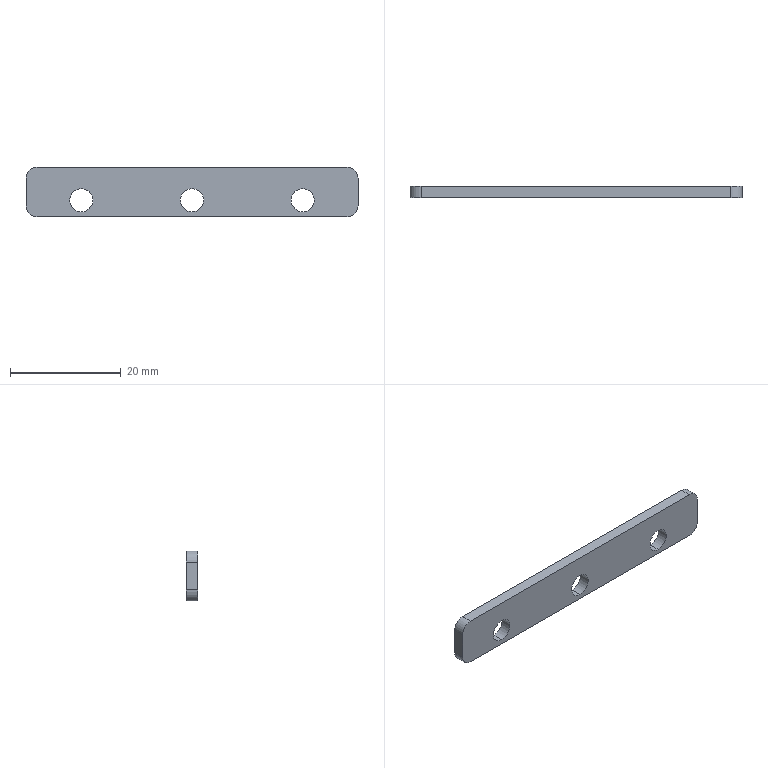Part | 1 solid | 16 faces | box 60 x 2 x 9 mm | volume 990.006 mm3 | cylinder 10 | plane 6 | commonest cylinder face diameters 4.2 x6 4 x4
STEP:
#1=CARTESIAN_POINT('',(-20.,-2.,-3.6));
#2=VERTEX_POINT('',#1);
#3=CARTESIAN_POINT('',(-20.,-2.,0.6));
#4=VERTEX_POINT('',#3);
#5=CARTESIAN_POINT('',(-20.,-2.,-1.5));
#6=DIRECTION('',(0.,1.,0.));
#7=DIRECTION('',(0.,0.,1.));
#8=AXIS2_PLACEMENT_3D('',#5,#6,#7);
#9=CIRCLE('',#8,2.1);
#10=EDGE_CURVE('',#2,#4,#9,.T.);
#11=ORIENTED_EDGE('',*,*,#10,.F.);
#12=CARTESIAN_POINT('',(-20.,0.,-3.6));
#13=VERTEX_POINT('',#12);
#14=CARTESIAN_POINT('',(-20.,-2.,-3.6));
#15=DIRECTION('',(0.,1.,0.));
#16=VECTOR('',#15,1000.);
#17=LINE('',#14,#16);
#18=EDGE_CURVE('',#2,#13,#17,.T.);
#19=ORIENTED_EDGE('',*,*,#18,.T.);
#20=CARTESIAN_POINT('',(-20.,0.,0.6));
#21=VERTEX_POINT('',#20);
#22=CARTESIAN_POINT('',(-20.,0.,-1.5));
#23=DIRECTION('',(0.,1.,0.));
#24=DIRECTION('',(0.,0.,1.));
#25=AXIS2_PLACEMENT_3D('',#22,#23,#24);
#26=CIRCLE('',#25,2.1);
#27=EDGE_CURVE('',#13,#21,#26,.T.);
#28=ORIENTED_EDGE('',*,*,#27,.T.);
#29=CARTESIAN_POINT('',(-20.,-2.,0.6));
#30=DIRECTION('',(0.,1.,0.));
#31=VECTOR('',#30,1000.);
#32=LINE('',#29,#31);
#33=EDGE_CURVE('',#4,#21,#32,.T.);
#34=ORIENTED_EDGE('',*,*,#33,.F.);
#35=EDGE_LOOP('',(#11,#19,#28,#34));
#36=FACE_OUTER_BOUND('',#35,.T.);
#37=CARTESIAN_POINT('',(-20.,-2.,-1.5));
#38=DIRECTION('',(0.,1.,0.));
#39=DIRECTION('',(0.,0.,1.));
#40=AXIS2_PLACEMENT_3D('',#37,#38,#39);
#41=CYLINDRICAL_SURFACE('',#40,2.1);
#42=ADVANCED_FACE('',(#36),#41,.F.);
#43=CARTESIAN_POINT('',(0.,-2.,-3.6));
#44=VERTEX_POINT('',#43);
#45=CARTESIAN_POINT('',(0.,-2.,0.6));
#46=VERTEX_POINT('',#45);
#47=CARTESIAN_POINT('',(0.,-2.,-1.5));
#48=DIRECTION('',(0.,1.,0.));
#49=DIRECTION('',(0.,0.,1.));
#50=AXIS2_PLACEMENT_3D('',#47,#48,#49);
#51=CIRCLE('',#50,2.1);
#52=EDGE_CURVE('',#44,#46,#51,.T.);
#53=ORIENTED_EDGE('',*,*,#52,.F.);
#54=CARTESIAN_POINT('',(0.,0.,-3.6));
#55=VERTEX_POINT('',#54);
#56=CARTESIAN_POINT('',(0.,-2.,-3.6));
#57=DIRECTION('',(0.,1.,0.));
#58=VECTOR('',#57,1000.);
#59=LINE('',#56,#58);
#60=EDGE_CURVE('',#44,#55,#59,.T.);
#61=ORIENTED_EDGE('',*,*,#60,.T.);
#62=CARTESIAN_POINT('',(0.,0.,0.6));
#63=VERTEX_POINT('',#62);
#64=CARTESIAN_POINT('',(0.,0.,-1.5));
#65=DIRECTION('',(0.,1.,0.));
#66=DIRECTION('',(0.,0.,1.));
#67=AXIS2_PLACEMENT_3D('',#64,#65,#66);
#68=CIRCLE('',#67,2.1);
#69=EDGE_CURVE('',#55,#63,#68,.T.);
#70=ORIENTED_EDGE('',*,*,#69,.T.);
#71=CARTESIAN_POINT('',(0.,-2.,0.6));
#72=DIRECTION('',(0.,1.,0.));
#73=VECTOR('',#72,1000.);
#74=LINE('',#71,#73);
#75=EDGE_CURVE('',#46,#63,#74,.T.);
#76=ORIENTED_EDGE('',*,*,#75,.F.);
#77=EDGE_LOOP('',(#53,#61,#70,#76));
#78=FACE_OUTER_BOUND('',#77,.T.);
#79=CARTESIAN_POINT('',(0.,-2.,-1.5));
#80=DIRECTION('',(0.,1.,0.));
#81=DIRECTION('',(0.,0.,1.));
#82=AXIS2_PLACEMENT_3D('',#79,#80,#81);
#83=CYLINDRICAL_SURFACE('',#82,2.1);
#84=ADVANCED_FACE('',(#78),#83,.F.);
#85=CARTESIAN_POINT('',(20.,-2.,-3.6));
#86=VERTEX_POINT('',#85);
#87=CARTESIAN_POINT('',(20.,-2.,0.6));
#88=VERTEX_POINT('',#87);
#89=CARTESIAN_POINT('',(20.,-2.,-1.5));
#90=DIRECTION('',(0.,1.,0.));
#91=DIRECTION('',(0.,0.,1.));
#92=AXIS2_PLACEMENT_3D('',#89,#90,#91);
#93=CIRCLE('',#92,2.1);
#94=EDGE_CURVE('',#86,#88,#93,.T.);
#95=ORIENTED_EDGE('',*,*,#94,.F.);
#96=CARTESIAN_POINT('',(20.,0.,-3.6));
#97=VERTEX_POINT('',#96);
#98=CARTESIAN_POINT('',(20.,-2.,-3.6));
#99=DIRECTION('',(0.,1.,0.));
#100=VECTOR('',#99,1000.);
#101=LINE('',#98,#100);
#102=EDGE_CURVE('',#86,#97,#101,.T.);
#103=ORIENTED_EDGE('',*,*,#102,.T.);
#104=CARTESIAN_POINT('',(20.,0.,0.6));
#105=VERTEX_POINT('',#104);
#106=CARTESIAN_POINT('',(20.,0.,-1.5));
#107=DIRECTION('',(0.,1.,0.));
#108=DIRECTION('',(0.,0.,1.));
#109=AXIS2_PLACEMENT_3D('',#106,#107,#108);
#110=CIRCLE('',#109,2.1);
#111=EDGE_CURVE('',#97,#105,#110,.T.);
#112=ORIENTED_EDGE('',*,*,#111,.T.);
#113=CARTESIAN_POINT('',(20.,-2.,0.6));
#114=DIRECTION('',(0.,1.,0.));
#115=VECTOR('',#114,1000.);
#116=LINE('',#113,#115);
#117=EDGE_CURVE('',#88,#105,#116,.T.);
#118=ORIENTED_EDGE('',*,*,#117,.F.);
#119=EDGE_LOOP('',(#95,#103,#112,#118));
#120=FACE_OUTER_BOUND('',#119,.T.);
#121=CARTESIAN_POINT('',(20.,-2.,-1.5));
#122=DIRECTION('',(0.,1.,0.));
#123=DIRECTION('',(0.,0.,1.));
#124=AXIS2_PLACEMENT_3D('',#121,#122,#123);
#125=CYLINDRICAL_SURFACE('',#124,2.1);
#126=ADVANCED_FACE('',(#120),#125,.F.);
#127=CARTESIAN_POINT('',(30.,0.,2.5));
#128=VERTEX_POINT('',#127);
#129=CARTESIAN_POINT('',(30.,0.,-2.5));
#130=VERTEX_POINT('',#129);
#131=CARTESIAN_POINT('',(30.,0.,4.5));
#132=DIRECTION('',(0.,0.,-1.));
#133=VECTOR('',#132,1000.);
#134=LINE('',#131,#133);
#135=EDGE_CURVE('',#128,#130,#134,.T.);
#136=ORIENTED_EDGE('',*,*,#135,.F.);
#137=CARTESIAN_POINT('',(30.,-2.,2.5));
#138=VERTEX_POINT('',#137);
#139=CARTESIAN_POINT('',(30.,-2.,2.5));
#140=DIRECTION('',(0.,-1.,0.));
#141=VECTOR('',#140,1000.);
#142=LINE('',#139,#141);
#143=EDGE_CURVE('',#128,#138,#142,.T.);
#144=ORIENTED_EDGE('',*,*,#143,.T.);
#145=CARTESIAN_POINT('',(30.,-2.,-2.5));
#146=VERTEX_POINT('',#145);
#147=CARTESIAN_POINT('',(30.,-2.,4.5));
#148=DIRECTION('',(0.,0.,-1.));
#149=VECTOR('',#148,1000.);
#150=LINE('',#147,#149);
#151=EDGE_CURVE('',#138,#146,#150,.T.);
#152=ORIENTED_EDGE('',*,*,#151,.T.);
#153=CARTESIAN_POINT('',(30.,-2.,-2.5));
#154=DIRECTION('',(0.,1.,0.));
#155=VECTOR('',#154,1000.);
#156=LINE('',#153,#155);
#157=EDGE_CURVE('',#146,#130,#156,.T.);
#158=ORIENTED_EDGE('',*,*,#157,.T.);
#159=EDGE_LOOP('',(#136,#144,#152,#158));
#160=FACE_OUTER_BOUND('',#159,.T.);
#161=CARTESIAN_POINT('',(30.,-2.,4.5));
#162=DIRECTION('',(1.,0.,0.));
#163=DIRECTION('',(0.,0.,-1.));
#164=AXIS2_PLACEMENT_3D('',#161,#162,#163);
#165=PLANE('',#164);
#166=ADVANCED_FACE('',(#160),#165,.T.);
#167=CARTESIAN_POINT('',(-28.,0.,4.5));
#168=VERTEX_POINT('',#167);
#169=CARTESIAN_POINT('',(28.,0.,4.5));
#170=VERTEX_POINT('',#169);
#171=CARTESIAN_POINT('',(-30.,0.,4.5));
#172=DIRECTION('',(1.,0.,0.));
#173=VECTOR('',#172,1000.);
#174=LINE('',#171,#173);
#175=EDGE_CURVE('',#168,#170,#174,.T.);
#176=ORIENTED_EDGE('',*,*,#175,.F.);
#177=CARTESIAN_POINT('',(-28.,-2.,4.5));
#178=VERTEX_POINT('',#177);
#179=CARTESIAN_POINT('',(-28.,-2.,4.5));
#180=DIRECTION('',(0.,-1.,0.));
#181=VECTOR('',#180,1000.);
#182=LINE('',#179,#181);
#183=EDGE_CURVE('',#168,#178,#182,.T.);
#184=ORIENTED_EDGE('',*,*,#183,.T.);
#185=CARTESIAN_POINT('',(28.,-2.,4.5));
#186=VERTEX_POINT('',#185);
#187=CARTESIAN_POINT('',(-30.,-2.,4.5));
#188=DIRECTION('',(1.,0.,0.));
#189=VECTOR('',#188,1000.);
#190=LINE('',#187,#189);
#191=EDGE_CURVE('',#178,#186,#190,.T.);
#192=ORIENTED_EDGE('',*,*,#191,.T.);
#193=CARTESIAN_POINT('',(28.,-2.,4.5));
#194=DIRECTION('',(0.,1.,0.));
#195=VECTOR('',#194,1000.);
#196=LINE('',#193,#195);
#197=EDGE_CURVE('',#186,#170,#196,.T.);
#198=ORIENTED_EDGE('',*,*,#197,.T.);
#199=EDGE_LOOP('',(#176,#184,#192,#198));
#200=FACE_OUTER_BOUND('',#199,.T.);
#201=CARTESIAN_POINT('',(-30.,-2.,4.5));
#202=DIRECTION('',(0.,0.,1.));
#203=DIRECTION('',(1.,0.,0.));
#204=AXIS2_PLACEMENT_3D('',#201,#202,#203);
#205=PLANE('',#204);
#206=ADVANCED_FACE('',(#200),#205,.T.);
#207=CARTESIAN_POINT('',(-30.,0.,-2.5));
#208=VERTEX_POINT('',#207);
#209=CARTESIAN_POINT('',(-30.,0.,2.5));
#210=VERTEX_POINT('',#209);
#211=CARTESIAN_POINT('',(-30.,0.,4.5));
#212=DIRECTION('',(0.,0.,1.));
#213=VECTOR('',#212,1000.);
#214=LINE('',#211,#213);
#215=EDGE_CURVE('',#208,#210,#214,.T.);
#216=ORIENTED_EDGE('',*,*,#215,.F.);
#217=CARTESIAN_POINT('',(-30.,-2.,-2.5));
#218=VERTEX_POINT('',#217);
#219=CARTESIAN_POINT('',(-30.,-2.,-2.5));
#220=DIRECTION('',(0.,-1.,0.));
#221=VECTOR('',#220,1000.);
#222=LINE('',#219,#221);
#223=EDGE_CURVE('',#208,#218,#222,.T.);
#224=ORIENTED_EDGE('',*,*,#223,.T.);
#225=CARTESIAN_POINT('',(-30.,-2.,2.5));
#226=VERTEX_POINT('',#225);
#227=CARTESIAN_POINT('',(-30.,-2.,4.5));
#228=DIRECTION('',(0.,0.,1.));
#229=VECTOR('',#228,1000.);
#230=LINE('',#227,#229);
#231=EDGE_CURVE('',#218,#226,#230,.T.);
#232=ORIENTED_EDGE('',*,*,#231,.T.);
#233=CARTESIAN_POINT('',(-30.,-2.,2.5));
#234=DIRECTION('',(0.,1.,0.));
#235=VECTOR('',#234,1000.);
#236=LINE('',#233,#235);
#237=EDGE_CURVE('',#226,#210,#236,.T.);
#238=ORIENTED_EDGE('',*,*,#237,.T.);
#239=EDGE_LOOP('',(#216,#224,#232,#238));
#240=FACE_OUTER_BOUND('',#239,.T.);
#241=CARTESIAN_POINT('',(-30.,-2.,4.5));
#242=DIRECTION('',(-1.,0.,0.));
#243=DIRECTION('',(0.,0.,1.));
#244=AXIS2_PLACEMENT_3D('',#241,#242,#243);
#245=PLANE('',#244);
#246=ADVANCED_FACE('',(#240),#245,.T.);
#247=CARTESIAN_POINT('',(28.,-2.,-4.5));
#248=VERTEX_POINT('',#247);
#249=CARTESIAN_POINT('',(-28.,-2.,-4.5));
#250=VERTEX_POINT('',#249);
#251=CARTESIAN_POINT('',(-30.,-2.,-4.5));
#252=DIRECTION('',(-1.,0.,0.));
#253=VECTOR('',#252,1000.);
#254=LINE('',#251,#253);
#255=EDGE_CURVE('',#248,#250,#254,.T.);
#256=ORIENTED_EDGE('',*,*,#255,.T.);
#257=CARTESIAN_POINT('',(-28.,0.,-4.5));
#258=VERTEX_POINT('',#257);
#259=CARTESIAN_POINT('',(-28.,-2.,-4.5));
#260=DIRECTION('',(0.,1.,0.));
#261=VECTOR('',#260,1000.);
#262=LINE('',#259,#261);
#263=EDGE_CURVE('',#250,#258,#262,.T.);
#264=ORIENTED_EDGE('',*,*,#263,.T.);
#265=CARTESIAN_POINT('',(28.,0.,-4.5));
#266=VERTEX_POINT('',#265);
#267=CARTESIAN_POINT('',(-30.,0.,-4.5));
#268=DIRECTION('',(-1.,0.,0.));
#269=VECTOR('',#268,1000.);
#270=LINE('',#267,#269);
#271=EDGE_CURVE('',#266,#258,#270,.T.);
#272=ORIENTED_EDGE('',*,*,#271,.F.);
#273=CARTESIAN_POINT('',(28.,-2.,-4.5));
#274=DIRECTION('',(0.,-1.,0.));
#275=VECTOR('',#274,1000.);
#276=LINE('',#273,#275);
#277=EDGE_CURVE('',#266,#248,#276,.T.);
#278=ORIENTED_EDGE('',*,*,#277,.T.);
#279=EDGE_LOOP('',(#256,#264,#272,#278));
#280=FACE_OUTER_BOUND('',#279,.T.);
#281=CARTESIAN_POINT('',(-30.,-2.,-4.5));
#282=DIRECTION('',(0.,0.,-1.));
#283=DIRECTION('',(-1.,0.,0.));
#284=AXIS2_PLACEMENT_3D('',#281,#282,#283);
#285=PLANE('',#284);
#286=ADVANCED_FACE('',(#280),#285,.T.);
#287=CARTESIAN_POINT('',(-20.,-2.,-1.5));
#288=DIRECTION('',(0.,1.,0.));
#289=DIRECTION('',(0.,0.,1.));
#290=AXIS2_PLACEMENT_3D('',#287,#288,#289);
#291=CIRCLE('',#290,2.1);
#292=EDGE_CURVE('',#4,#2,#291,.T.);
#293=ORIENTED_EDGE('',*,*,#292,.T.);
#294=ORIENTED_EDGE('',*,*,#10,.T.);
#295=EDGE_LOOP('',(#293,#294));
#296=FACE_BOUND('',#295,.T.);
#297=CARTESIAN_POINT('',(0.,-2.,-1.5));
#298=DIRECTION('',(0.,1.,0.));
#299=DIRECTION('',(0.,0.,1.));
#300=AXIS2_PLACEMENT_3D('',#297,#298,#299);
#301=CIRCLE('',#300,2.1);
#302=EDGE_CURVE('',#46,#44,#301,.T.);
#303=ORIENTED_EDGE('',*,*,#302,.T.);
#304=ORIENTED_EDGE('',*,*,#52,.T.);
#305=EDGE_LOOP('',(#303,#304));
#306=FACE_BOUND('',#305,.T.);
#307=CARTESIAN_POINT('',(20.,-2.,-1.5));
#308=DIRECTION('',(0.,1.,0.));
#309=DIRECTION('',(0.,0.,1.));
#310=AXIS2_PLACEMENT_3D('',#307,#308,#309);
#311=CIRCLE('',#310,2.1);
#312=EDGE_CURVE('',#88,#86,#311,.T.);
#313=ORIENTED_EDGE('',*,*,#312,.T.);
#314=ORIENTED_EDGE('',*,*,#94,.T.);
#315=EDGE_LOOP('',(#313,#314));
#316=FACE_BOUND('',#315,.T.);
#317=ORIENTED_EDGE('',*,*,#231,.F.);
#318=CARTESIAN_POINT('',(-28.,-2.,-2.5));
#319=DIRECTION('',(0.,-1.,0.));
#320=DIRECTION('',(0.,0.,-1.));
#321=AXIS2_PLACEMENT_3D('',#318,#319,#320);
#322=CIRCLE('',#321,2.);
#323=EDGE_CURVE('',#218,#250,#322,.T.);
#324=ORIENTED_EDGE('',*,*,#323,.T.);
#325=ORIENTED_EDGE('',*,*,#255,.F.);
#326=CARTESIAN_POINT('',(28.,-2.,-2.5));
#327=DIRECTION('',(0.,-1.,0.));
#328=DIRECTION('',(0.,0.,-1.));
#329=AXIS2_PLACEMENT_3D('',#326,#327,#328);
#330=CIRCLE('',#329,2.);
#331=EDGE_CURVE('',#248,#146,#330,.T.);
#332=ORIENTED_EDGE('',*,*,#331,.T.);
#333=ORIENTED_EDGE('',*,*,#151,.F.);
#334=CARTESIAN_POINT('',(28.,-2.,2.5));
#335=DIRECTION('',(0.,-1.,0.));
#336=DIRECTION('',(0.,0.,-1.));
#337=AXIS2_PLACEMENT_3D('',#334,#335,#336);
#338=CIRCLE('',#337,2.);
#339=EDGE_CURVE('',#138,#186,#338,.T.);
#340=ORIENTED_EDGE('',*,*,#339,.T.);
#341=ORIENTED_EDGE('',*,*,#191,.F.);
#342=CARTESIAN_POINT('',(-28.,-2.,2.5));
#343=DIRECTION('',(0.,-1.,0.));
#344=DIRECTION('',(0.,0.,-1.));
#345=AXIS2_PLACEMENT_3D('',#342,#343,#344);
#346=CIRCLE('',#345,2.);
#347=EDGE_CURVE('',#178,#226,#346,.T.);
#348=ORIENTED_EDGE('',*,*,#347,.T.);
#349=EDGE_LOOP('',(#317,#324,#325,#332,#333,#340,#341,#348));
#350=FACE_OUTER_BOUND('',#349,.T.);
#351=CARTESIAN_POINT('',(0.,-2.,0.));
#352=DIRECTION('',(0.,-1.,0.));
#353=DIRECTION('',(0.,0.,-1.));
#354=AXIS2_PLACEMENT_3D('',#351,#352,#353);
#355=PLANE('',#354);
#356=ADVANCED_FACE('',(#296,#306,#316,#350),#355,.T.);
#357=CARTESIAN_POINT('',(-20.,0.,-1.5));
#358=DIRECTION('',(0.,1.,0.));
#359=DIRECTION('',(0.,0.,1.));
#360=AXIS2_PLACEMENT_3D('',#357,#358,#359);
#361=CIRCLE('',#360,2.1);
#362=EDGE_CURVE('',#21,#13,#361,.T.);
#363=ORIENTED_EDGE('',*,*,#362,.F.);
#364=ORIENTED_EDGE('',*,*,#27,.F.);
#365=EDGE_LOOP('',(#363,#364));
#366=FACE_BOUND('',#365,.T.);
#367=CARTESIAN_POINT('',(0.,0.,-1.5));
#368=DIRECTION('',(0.,1.,0.));
#369=DIRECTION('',(0.,0.,1.));
#370=AXIS2_PLACEMENT_3D('',#367,#368,#369);
#371=CIRCLE('',#370,2.1);
#372=EDGE_CURVE('',#63,#55,#371,.T.);
#373=ORIENTED_EDGE('',*,*,#372,.F.);
#374=ORIENTED_EDGE('',*,*,#69,.F.);
#375=EDGE_LOOP('',(#373,#374));
#376=FACE_BOUND('',#375,.T.);
#377=CARTESIAN_POINT('',(20.,0.,-1.5));
#378=DIRECTION('',(0.,1.,0.));
#379=DIRECTION('',(0.,0.,1.));
#380=AXIS2_PLACEMENT_3D('',#377,#378,#379);
#381=CIRCLE('',#380,2.1);
#382=EDGE_CURVE('',#105,#97,#381,.T.);
#383=ORIENTED_EDGE('',*,*,#382,.F.);
#384=ORIENTED_EDGE('',*,*,#111,.F.);
#385=EDGE_LOOP('',(#383,#384));
#386=FACE_BOUND('',#385,.T.);
#387=ORIENTED_EDGE('',*,*,#271,.T.);
#388=CARTESIAN_POINT('',(-28.,0.,-2.5));
#389=DIRECTION('',(0.,1.,0.));
#390=DIRECTION('',(0.,0.,-1.));
#391=AXIS2_PLACEMENT_3D('',#388,#389,#390);
#392=CIRCLE('',#391,2.);
#393=EDGE_CURVE('',#258,#208,#392,.T.);
#394=ORIENTED_EDGE('',*,*,#393,.T.);
#395=ORIENTED_EDGE('',*,*,#215,.T.);
#396=CARTESIAN_POINT('',(-28.,0.,2.5));
#397=DIRECTION('',(0.,1.,0.));
#398=DIRECTION('',(0.,0.,-1.));
#399=AXIS2_PLACEMENT_3D('',#396,#397,#398);
#400=CIRCLE('',#399,2.);
#401=EDGE_CURVE('',#210,#168,#400,.T.);
#402=ORIENTED_EDGE('',*,*,#401,.T.);
#403=ORIENTED_EDGE('',*,*,#175,.T.);
#404=CARTESIAN_POINT('',(28.,0.,2.5));
#405=DIRECTION('',(0.,1.,0.));
#406=DIRECTION('',(0.,0.,-1.));
#407=AXIS2_PLACEMENT_3D('',#404,#405,#406);
#408=CIRCLE('',#407,2.);
#409=EDGE_CURVE('',#170,#128,#408,.T.);
#410=ORIENTED_EDGE('',*,*,#409,.T.);
#411=ORIENTED_EDGE('',*,*,#135,.T.);
#412=CARTESIAN_POINT('',(28.,0.,-2.5));
#413=DIRECTION('',(0.,1.,0.));
#414=DIRECTION('',(0.,0.,-1.));
#415=AXIS2_PLACEMENT_3D('',#412,#413,#414);
#416=CIRCLE('',#415,2.);
#417=EDGE_CURVE('',#130,#266,#416,.T.);
#418=ORIENTED_EDGE('',*,*,#417,.T.);
#419=EDGE_LOOP('',(#387,#394,#395,#402,#403,#410,#411,#418));
#420=FACE_OUTER_BOUND('',#419,.T.);
#421=CARTESIAN_POINT('',(0.,0.,0.));
#422=DIRECTION('',(0.,-1.,0.));
#423=DIRECTION('',(0.,0.,-1.));
#424=AXIS2_PLACEMENT_3D('',#421,#422,#423);
#425=PLANE('',#424);
#426=ADVANCED_FACE('',(#366,#376,#386,#420),#425,.F.);
#427=ORIENTED_EDGE('',*,*,#102,.F.);
#428=ORIENTED_EDGE('',*,*,#312,.F.);
#429=ORIENTED_EDGE('',*,*,#117,.T.);
#430=ORIENTED_EDGE('',*,*,#382,.T.);
#431=EDGE_LOOP('',(#427,#428,#429,#430));
#432=FACE_OUTER_BOUND('',#431,.T.);
#433=CARTESIAN_POINT('',(20.,-2.,-1.5));
#434=DIRECTION('',(0.,1.,0.));
#435=DIRECTION('',(0.,0.,1.));
#436=AXIS2_PLACEMENT_3D('',#433,#434,#435);
#437=CYLINDRICAL_SURFACE('',#436,2.1);
#438=ADVANCED_FACE('',(#432),#437,.F.);
#439=ORIENTED_EDGE('',*,*,#60,.F.);
#440=ORIENTED_EDGE('',*,*,#302,.F.);
#441=ORIENTED_EDGE('',*,*,#75,.T.);
#442=ORIENTED_EDGE('',*,*,#372,.T.);
#443=EDGE_LOOP('',(#439,#440,#441,#442));
#444=FACE_OUTER_BOUND('',#443,.T.);
#445=CARTESIAN_POINT('',(0.,-2.,-1.5));
#446=DIRECTION('',(0.,1.,0.));
#447=DIRECTION('',(0.,0.,1.));
#448=AXIS2_PLACEMENT_3D('',#445,#446,#447);
#449=CYLINDRICAL_SURFACE('',#448,2.1);
#450=ADVANCED_FACE('',(#444),#449,.F.);
#451=ORIENTED_EDGE('',*,*,#18,.F.);
#452=ORIENTED_EDGE('',*,*,#292,.F.);
#453=ORIENTED_EDGE('',*,*,#33,.T.);
#454=ORIENTED_EDGE('',*,*,#362,.T.);
#455=EDGE_LOOP('',(#451,#452,#453,#454));
#456=FACE_OUTER_BOUND('',#455,.T.);
#457=CARTESIAN_POINT('',(-20.,-2.,-1.5));
#458=DIRECTION('',(0.,1.,0.));
#459=DIRECTION('',(0.,0.,1.));
#460=AXIS2_PLACEMENT_3D('',#457,#458,#459);
#461=CYLINDRICAL_SURFACE('',#460,2.1);
#462=ADVANCED_FACE('',(#456),#461,.F.);
#463=ORIENTED_EDGE('',*,*,#323,.F.);
#464=ORIENTED_EDGE('',*,*,#223,.F.);
#465=ORIENTED_EDGE('',*,*,#393,.F.);
#466=ORIENTED_EDGE('',*,*,#263,.F.);
#467=EDGE_LOOP('',(#463,#464,#465,#466));
#468=FACE_OUTER_BOUND('',#467,.T.);
#469=CARTESIAN_POINT('',(-28.,-2.,-2.5));
#470=DIRECTION('',(0.,1.,0.));
#471=DIRECTION('',(0.,0.,1.));
#472=AXIS2_PLACEMENT_3D('',#469,#470,#471);
#473=CYLINDRICAL_SURFACE('',#472,2.);
#474=ADVANCED_FACE('',(#468),#473,.T.);
#475=ORIENTED_EDGE('',*,*,#347,.F.);
#476=ORIENTED_EDGE('',*,*,#183,.F.);
#477=ORIENTED_EDGE('',*,*,#401,.F.);
#478=ORIENTED_EDGE('',*,*,#237,.F.);
#479=EDGE_LOOP('',(#475,#476,#477,#478));
#480=FACE_OUTER_BOUND('',#479,.T.);
#481=CARTESIAN_POINT('',(-28.,-2.,2.5));
#482=DIRECTION('',(0.,1.,0.));
#483=DIRECTION('',(0.,0.,1.));
#484=AXIS2_PLACEMENT_3D('',#481,#482,#483);
#485=CYLINDRICAL_SURFACE('',#484,2.);
#486=ADVANCED_FACE('',(#480),#485,.T.);
#487=ORIENTED_EDGE('',*,*,#339,.F.);
#488=ORIENTED_EDGE('',*,*,#143,.F.);
#489=ORIENTED_EDGE('',*,*,#409,.F.);
#490=ORIENTED_EDGE('',*,*,#197,.F.);
#491=EDGE_LOOP('',(#487,#488,#489,#490));
#492=FACE_OUTER_BOUND('',#491,.T.);
#493=CARTESIAN_POINT('',(28.,-2.,2.5));
#494=DIRECTION('',(0.,1.,0.));
#495=DIRECTION('',(0.,0.,1.));
#496=AXIS2_PLACEMENT_3D('',#493,#494,#495);
#497=CYLINDRICAL_SURFACE('',#496,2.);
#498=ADVANCED_FACE('',(#492),#497,.T.);
#499=ORIENTED_EDGE('',*,*,#331,.F.);
#500=ORIENTED_EDGE('',*,*,#277,.F.);
#501=ORIENTED_EDGE('',*,*,#417,.F.);
#502=ORIENTED_EDGE('',*,*,#157,.F.);
#503=EDGE_LOOP('',(#499,#500,#501,#502));
#504=FACE_OUTER_BOUND('',#503,.T.);
#505=CARTESIAN_POINT('',(28.,-2.,-2.5));
#506=DIRECTION('',(0.,1.,0.));
#507=DIRECTION('',(0.,0.,1.));
#508=AXIS2_PLACEMENT_3D('',#505,#506,#507);
#509=CYLINDRICAL_SURFACE('',#508,2.);
#510=ADVANCED_FACE('',(#504),#509,.T.);
#511=CLOSED_SHELL('',(#42,#84,#126,#166,#206,#246,#286,#356,#426,#438,#450,#462,#474,#486,#498,#510));
#512=MANIFOLD_SOLID_BREP('',#511);
#513=CARTESIAN_POINT('',(0.,0.,0.));
#514=DIRECTION('',(0.,0.,1.));
#515=DIRECTION('',(1.,0.,0.));
#516=AXIS2_PLACEMENT_3D('',#513,#514,#515);
#517=(LENGTH_UNIT()NAMED_UNIT(*)SI_UNIT(.MILLI.,.METRE.));
#518=UNCERTAINTY_MEASURE_WITH_UNIT(LENGTH_MEASURE(0.00001),#517,'','');
#519=(NAMED_UNIT(*)PLANE_ANGLE_UNIT()SI_UNIT($,.RADIAN.));
#520=(NAMED_UNIT(*)SI_UNIT($,.STERADIAN.)SOLID_ANGLE_UNIT());
#521=(GEOMETRIC_REPRESENTATION_CONTEXT(3)GLOBAL_UNCERTAINTY_ASSIGNED_CONTEXT((#518))GLOBAL_UNIT_ASSIGNED_CONTEXT((#517,#519,#520))REPRESENTATION_CONTEXT('',''));
#522=ADVANCED_BREP_SHAPE_REPRESENTATION('',(#512,#516),#521);